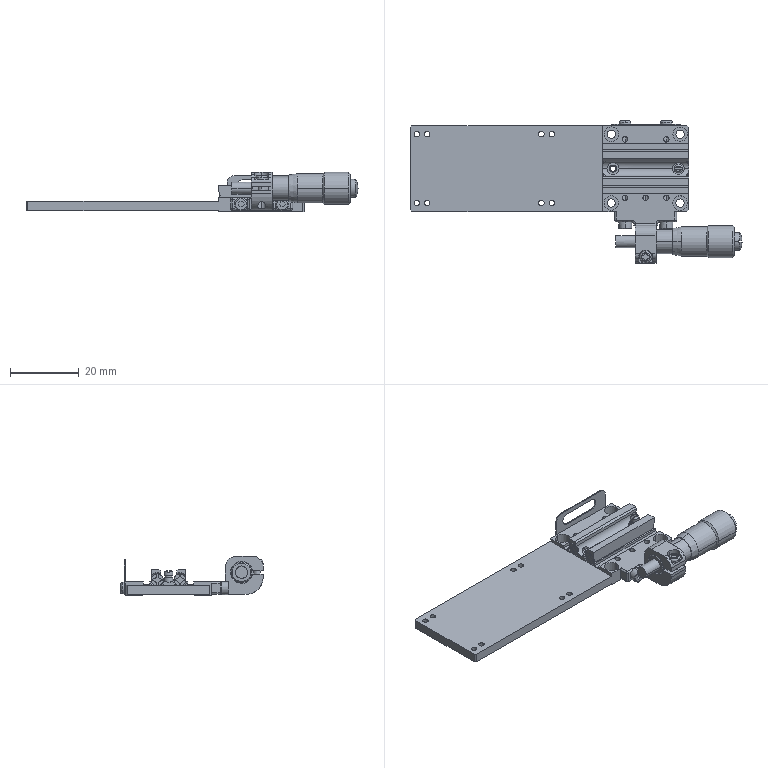Part | SolidWorks | features ICE 5, HoleWzd 3, MoveFace 3, BaseBody 1, Chamfer 1, Cut 1, DelFace 1 | 1 solid | 615 faces | box 96.495 x 41.4 x 11.45 mm | volume 8301 mm3 | plane 242 | cylinder 233 | cone 119 | torus 10 | sphere 7 | spline 4 | commonest cylinder face diameters 1.6 x46 1.567 x32 2 x32 2.4 x20 3.5 x20 1 x17